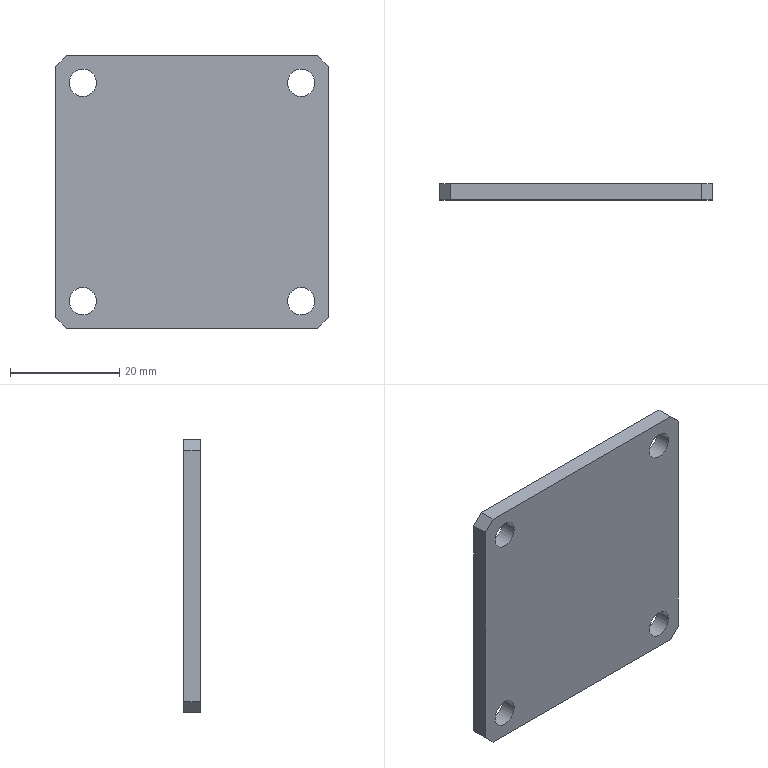Part | NX | 1 solid | 14 faces | box 50 x 3 x 50 mm | volume 7240 mm3 | plane 10 | cylinder 4 | commonest cylinder face diameters 5 x4
STEP:
#1=CARTESIAN_POINT('',(25.,3.,23.));
#2=VERTEX_POINT('',#1);
#3=CARTESIAN_POINT('',(25.,3.,-23.));
#4=VERTEX_POINT('',#3);
#5=CARTESIAN_POINT('',(25.,3.,25.));
#6=DIRECTION('',(0.,0.,-1.));
#7=VECTOR('',#6,1000.);
#8=LINE('',#5,#7);
#9=EDGE_CURVE('',#2,#4,#8,.T.);
#10=ORIENTED_EDGE('',*,*,#9,.F.);
#11=CARTESIAN_POINT('',(25.,0.,23.));
#12=VERTEX_POINT('',#11);
#13=CARTESIAN_POINT('',(25.,3.,23.));
#14=DIRECTION('',(0.,-1.,0.));
#15=VECTOR('',#14,1000.);
#16=LINE('',#13,#15);
#17=EDGE_CURVE('',#2,#12,#16,.T.);
#18=ORIENTED_EDGE('',*,*,#17,.T.);
#19=CARTESIAN_POINT('',(25.,0.,-23.));
#20=VERTEX_POINT('',#19);
#21=CARTESIAN_POINT('',(25.,0.,25.));
#22=DIRECTION('',(0.,0.,-1.));
#23=VECTOR('',#22,1000.);
#24=LINE('',#21,#23);
#25=EDGE_CURVE('',#12,#20,#24,.T.);
#26=ORIENTED_EDGE('',*,*,#25,.T.);
#27=CARTESIAN_POINT('',(25.,3.,-23.));
#28=DIRECTION('',(0.,1.,0.));
#29=VECTOR('',#28,1000.);
#30=LINE('',#27,#29);
#31=EDGE_CURVE('',#20,#4,#30,.T.);
#32=ORIENTED_EDGE('',*,*,#31,.T.);
#33=EDGE_LOOP('',(#10,#18,#26,#32));
#34=FACE_BOUND('',#33,.T.);
#35=CARTESIAN_POINT('',(25.,3.,25.));
#36=DIRECTION('',(-1.,0.,0.));
#37=DIRECTION('',(0.,0.,1.));
#38=AXIS2_PLACEMENT_3D('',#35,#36,#37);
#39=PLANE('',#38);
#40=ADVANCED_FACE('',(#34),#39,.F.);
#41=CARTESIAN_POINT('',(23.,3.,-25.));
#42=VERTEX_POINT('',#41);
#43=CARTESIAN_POINT('',(-23.,3.,-25.));
#44=VERTEX_POINT('',#43);
#45=CARTESIAN_POINT('',(-25.,3.,-25.));
#46=DIRECTION('',(-1.,0.,0.));
#47=VECTOR('',#46,1000.);
#48=LINE('',#45,#47);
#49=EDGE_CURVE('',#42,#44,#48,.T.);
#50=ORIENTED_EDGE('',*,*,#49,.F.);
#51=CARTESIAN_POINT('',(23.,0.,-25.));
#52=VERTEX_POINT('',#51);
#53=CARTESIAN_POINT('',(23.,3.,-25.));
#54=DIRECTION('',(0.,-1.,0.));
#55=VECTOR('',#54,1000.);
#56=LINE('',#53,#55);
#57=EDGE_CURVE('',#42,#52,#56,.T.);
#58=ORIENTED_EDGE('',*,*,#57,.T.);
#59=CARTESIAN_POINT('',(-23.,0.,-25.));
#60=VERTEX_POINT('',#59);
#61=CARTESIAN_POINT('',(-25.,0.,-25.));
#62=DIRECTION('',(-1.,0.,0.));
#63=VECTOR('',#62,1000.);
#64=LINE('',#61,#63);
#65=EDGE_CURVE('',#52,#60,#64,.T.);
#66=ORIENTED_EDGE('',*,*,#65,.T.);
#67=CARTESIAN_POINT('',(-23.,3.,-25.));
#68=DIRECTION('',(0.,1.,0.));
#69=VECTOR('',#68,1000.);
#70=LINE('',#67,#69);
#71=EDGE_CURVE('',#60,#44,#70,.T.);
#72=ORIENTED_EDGE('',*,*,#71,.T.);
#73=EDGE_LOOP('',(#50,#58,#66,#72));
#74=FACE_BOUND('',#73,.T.);
#75=CARTESIAN_POINT('',(-25.,3.,-25.));
#76=DIRECTION('',(0.,0.,1.));
#77=DIRECTION('',(1.,0.,0.));
#78=AXIS2_PLACEMENT_3D('',#75,#76,#77);
#79=PLANE('',#78);
#80=ADVANCED_FACE('',(#74),#79,.F.);
#81=CARTESIAN_POINT('',(-25.,0.,-23.));
#82=VERTEX_POINT('',#81);
#83=CARTESIAN_POINT('',(-25.,0.,23.));
#84=VERTEX_POINT('',#83);
#85=CARTESIAN_POINT('',(-25.,0.,25.));
#86=DIRECTION('',(0.,0.,1.));
#87=VECTOR('',#86,1000.);
#88=LINE('',#85,#87);
#89=EDGE_CURVE('',#82,#84,#88,.T.);
#90=ORIENTED_EDGE('',*,*,#89,.T.);
#91=CARTESIAN_POINT('',(-25.,3.,23.));
#92=VERTEX_POINT('',#91);
#93=CARTESIAN_POINT('',(-25.,3.,23.));
#94=DIRECTION('',(0.,1.,0.));
#95=VECTOR('',#94,1000.);
#96=LINE('',#93,#95);
#97=EDGE_CURVE('',#84,#92,#96,.T.);
#98=ORIENTED_EDGE('',*,*,#97,.T.);
#99=CARTESIAN_POINT('',(-25.,3.,-23.));
#100=VERTEX_POINT('',#99);
#101=CARTESIAN_POINT('',(-25.,3.,25.));
#102=DIRECTION('',(0.,0.,1.));
#103=VECTOR('',#102,1000.);
#104=LINE('',#101,#103);
#105=EDGE_CURVE('',#100,#92,#104,.T.);
#106=ORIENTED_EDGE('',*,*,#105,.F.);
#107=CARTESIAN_POINT('',(-25.,3.,-23.));
#108=DIRECTION('',(0.,-1.,0.));
#109=VECTOR('',#108,1000.);
#110=LINE('',#107,#109);
#111=EDGE_CURVE('',#100,#82,#110,.T.);
#112=ORIENTED_EDGE('',*,*,#111,.T.);
#113=EDGE_LOOP('',(#90,#98,#106,#112));
#114=FACE_BOUND('',#113,.T.);
#115=CARTESIAN_POINT('',(-25.,3.,25.));
#116=DIRECTION('',(1.,0.,0.));
#117=DIRECTION('',(0.,0.,-1.));
#118=AXIS2_PLACEMENT_3D('',#115,#116,#117);
#119=PLANE('',#118);
#120=ADVANCED_FACE('',(#114),#119,.F.);
#121=CARTESIAN_POINT('',(-23.,3.,25.));
#122=VERTEX_POINT('',#121);
#123=CARTESIAN_POINT('',(23.,3.,25.));
#124=VERTEX_POINT('',#123);
#125=CARTESIAN_POINT('',(-25.,3.,25.));
#126=DIRECTION('',(1.,0.,0.));
#127=VECTOR('',#126,1000.);
#128=LINE('',#125,#127);
#129=EDGE_CURVE('',#122,#124,#128,.T.);
#130=ORIENTED_EDGE('',*,*,#129,.F.);
#131=CARTESIAN_POINT('',(-23.,0.,25.));
#132=VERTEX_POINT('',#131);
#133=CARTESIAN_POINT('',(-23.,3.,25.));
#134=DIRECTION('',(0.,-1.,0.));
#135=VECTOR('',#134,1000.);
#136=LINE('',#133,#135);
#137=EDGE_CURVE('',#122,#132,#136,.T.);
#138=ORIENTED_EDGE('',*,*,#137,.T.);
#139=CARTESIAN_POINT('',(23.,0.,25.));
#140=VERTEX_POINT('',#139);
#141=CARTESIAN_POINT('',(-25.,0.,25.));
#142=DIRECTION('',(1.,0.,0.));
#143=VECTOR('',#142,1000.);
#144=LINE('',#141,#143);
#145=EDGE_CURVE('',#132,#140,#144,.T.);
#146=ORIENTED_EDGE('',*,*,#145,.T.);
#147=CARTESIAN_POINT('',(23.,3.,25.));
#148=DIRECTION('',(0.,1.,0.));
#149=VECTOR('',#148,1000.);
#150=LINE('',#147,#149);
#151=EDGE_CURVE('',#140,#124,#150,.T.);
#152=ORIENTED_EDGE('',*,*,#151,.T.);
#153=EDGE_LOOP('',(#130,#138,#146,#152));
#154=FACE_BOUND('',#153,.T.);
#155=CARTESIAN_POINT('',(-25.,3.,25.));
#156=DIRECTION('',(0.,0.,-1.));
#157=DIRECTION('',(-1.,0.,0.));
#158=AXIS2_PLACEMENT_3D('',#155,#156,#157);
#159=PLANE('',#158);
#160=ADVANCED_FACE('',(#154),#159,.F.);
#161=CARTESIAN_POINT('',(-20.,3.,-17.5));
#162=VERTEX_POINT('',#161);
#163=CARTESIAN_POINT('',(-20.,3.,-20.));
#164=DIRECTION('',(0.,1.,0.));
#165=DIRECTION('',(0.,0.,1.));
#166=AXIS2_PLACEMENT_3D('',#163,#164,#165);
#167=CIRCLE('',#166,2.5);
#168=EDGE_CURVE('',#162,#162,#167,.T.);
#169=ORIENTED_EDGE('',*,*,#168,.F.);
#170=EDGE_LOOP('',(#169));
#171=FACE_BOUND('',#170,.T.);
#172=CARTESIAN_POINT('',(20.,3.,-17.5));
#173=VERTEX_POINT('',#172);
#174=CARTESIAN_POINT('',(20.,3.,-20.));
#175=DIRECTION('',(0.,1.,0.));
#176=DIRECTION('',(0.,0.,1.));
#177=AXIS2_PLACEMENT_3D('',#174,#175,#176);
#178=CIRCLE('',#177,2.5);
#179=EDGE_CURVE('',#173,#173,#178,.T.);
#180=ORIENTED_EDGE('',*,*,#179,.F.);
#181=EDGE_LOOP('',(#180));
#182=FACE_BOUND('',#181,.T.);
#183=CARTESIAN_POINT('',(20.,3.,22.5));
#184=VERTEX_POINT('',#183);
#185=CARTESIAN_POINT('',(20.,3.,20.));
#186=DIRECTION('',(0.,1.,0.));
#187=DIRECTION('',(0.,0.,1.));
#188=AXIS2_PLACEMENT_3D('',#185,#186,#187);
#189=CIRCLE('',#188,2.5);
#190=EDGE_CURVE('',#184,#184,#189,.T.);
#191=ORIENTED_EDGE('',*,*,#190,.F.);
#192=EDGE_LOOP('',(#191));
#193=FACE_BOUND('',#192,.T.);
#194=CARTESIAN_POINT('',(-20.,3.,22.5));
#195=VERTEX_POINT('',#194);
#196=CARTESIAN_POINT('',(-20.,3.,20.));
#197=DIRECTION('',(0.,1.,0.));
#198=DIRECTION('',(0.,0.,1.));
#199=AXIS2_PLACEMENT_3D('',#196,#197,#198);
#200=CIRCLE('',#199,2.5);
#201=EDGE_CURVE('',#195,#195,#200,.T.);
#202=ORIENTED_EDGE('',*,*,#201,.F.);
#203=EDGE_LOOP('',(#202));
#204=FACE_BOUND('',#203,.T.);
#205=ORIENTED_EDGE('',*,*,#105,.T.);
#206=CARTESIAN_POINT('',(-23.,3.,25.));
#207=DIRECTION('',(-0.7071,0.,-0.7071));
#208=VECTOR('',#207,1000.);
#209=LINE('',#206,#208);
#210=EDGE_CURVE('',#92,#122,#209,.F.);
#211=ORIENTED_EDGE('',*,*,#210,.T.);
#212=ORIENTED_EDGE('',*,*,#129,.T.);
#213=CARTESIAN_POINT('',(25.,3.,23.));
#214=DIRECTION('',(-0.7071,0.,0.7071));
#215=VECTOR('',#214,1000.);
#216=LINE('',#213,#215);
#217=EDGE_CURVE('',#124,#2,#216,.F.);
#218=ORIENTED_EDGE('',*,*,#217,.T.);
#219=ORIENTED_EDGE('',*,*,#9,.T.);
#220=CARTESIAN_POINT('',(23.,3.,-25.));
#221=DIRECTION('',(0.7071,0.,0.7071));
#222=VECTOR('',#221,1000.);
#223=LINE('',#220,#222);
#224=EDGE_CURVE('',#4,#42,#223,.F.);
#225=ORIENTED_EDGE('',*,*,#224,.T.);
#226=ORIENTED_EDGE('',*,*,#49,.T.);
#227=CARTESIAN_POINT('',(-25.,3.,-23.));
#228=DIRECTION('',(0.7071,0.,-0.7071));
#229=VECTOR('',#228,1000.);
#230=LINE('',#227,#229);
#231=EDGE_CURVE('',#44,#100,#230,.F.);
#232=ORIENTED_EDGE('',*,*,#231,.T.);
#233=EDGE_LOOP('',(#205,#211,#212,#218,#219,#225,#226,#232));
#234=FACE_BOUND('',#233,.T.);
#235=CARTESIAN_POINT('',(0.,3.,0.));
#236=DIRECTION('',(0.,-1.,0.));
#237=DIRECTION('',(0.,0.,-1.));
#238=AXIS2_PLACEMENT_3D('',#235,#236,#237);
#239=PLANE('',#238);
#240=ADVANCED_FACE('',(#171,#182,#193,#204,#234),#239,.F.);
#241=CARTESIAN_POINT('',(-20.,0.,-17.5));
#242=VERTEX_POINT('',#241);
#243=CARTESIAN_POINT('',(-20.,0.,-20.));
#244=DIRECTION('',(0.,1.,0.));
#245=DIRECTION('',(0.,0.,1.));
#246=AXIS2_PLACEMENT_3D('',#243,#244,#245);
#247=CIRCLE('',#246,2.5);
#248=EDGE_CURVE('',#242,#242,#247,.T.);
#249=ORIENTED_EDGE('',*,*,#248,.T.);
#250=EDGE_LOOP('',(#249));
#251=FACE_BOUND('',#250,.T.);
#252=CARTESIAN_POINT('',(20.,0.,-17.5));
#253=VERTEX_POINT('',#252);
#254=CARTESIAN_POINT('',(20.,0.,-20.));
#255=DIRECTION('',(0.,1.,0.));
#256=DIRECTION('',(0.,0.,1.));
#257=AXIS2_PLACEMENT_3D('',#254,#255,#256);
#258=CIRCLE('',#257,2.5);
#259=EDGE_CURVE('',#253,#253,#258,.T.);
#260=ORIENTED_EDGE('',*,*,#259,.T.);
#261=EDGE_LOOP('',(#260));
#262=FACE_BOUND('',#261,.T.);
#263=CARTESIAN_POINT('',(20.,0.,22.5));
#264=VERTEX_POINT('',#263);
#265=CARTESIAN_POINT('',(20.,0.,20.));
#266=DIRECTION('',(0.,1.,0.));
#267=DIRECTION('',(0.,0.,1.));
#268=AXIS2_PLACEMENT_3D('',#265,#266,#267);
#269=CIRCLE('',#268,2.5);
#270=EDGE_CURVE('',#264,#264,#269,.T.);
#271=ORIENTED_EDGE('',*,*,#270,.T.);
#272=EDGE_LOOP('',(#271));
#273=FACE_BOUND('',#272,.T.);
#274=CARTESIAN_POINT('',(-20.,0.,22.5));
#275=VERTEX_POINT('',#274);
#276=CARTESIAN_POINT('',(-20.,0.,20.));
#277=DIRECTION('',(0.,1.,0.));
#278=DIRECTION('',(0.,0.,1.));
#279=AXIS2_PLACEMENT_3D('',#276,#277,#278);
#280=CIRCLE('',#279,2.5);
#281=EDGE_CURVE('',#275,#275,#280,.T.);
#282=ORIENTED_EDGE('',*,*,#281,.T.);
#283=EDGE_LOOP('',(#282));
#284=FACE_BOUND('',#283,.T.);
#285=ORIENTED_EDGE('',*,*,#145,.F.);
#286=CARTESIAN_POINT('',(-24.,0.,24.));
#287=DIRECTION('',(0.7071,0.,0.7071));
#288=VECTOR('',#287,1000.);
#289=LINE('',#286,#288);
#290=EDGE_CURVE('',#132,#84,#289,.F.);
#291=ORIENTED_EDGE('',*,*,#290,.T.);
#292=ORIENTED_EDGE('',*,*,#89,.F.);
#293=CARTESIAN_POINT('',(-24.,0.,-24.));
#294=DIRECTION('',(-0.7071,0.,0.7071));
#295=VECTOR('',#294,1000.);
#296=LINE('',#293,#295);
#297=EDGE_CURVE('',#82,#60,#296,.F.);
#298=ORIENTED_EDGE('',*,*,#297,.T.);
#299=ORIENTED_EDGE('',*,*,#65,.F.);
#300=CARTESIAN_POINT('',(24.,0.,-24.));
#301=DIRECTION('',(-0.7071,0.,-0.7071));
#302=VECTOR('',#301,1000.);
#303=LINE('',#300,#302);
#304=EDGE_CURVE('',#52,#20,#303,.F.);
#305=ORIENTED_EDGE('',*,*,#304,.T.);
#306=ORIENTED_EDGE('',*,*,#25,.F.);
#307=CARTESIAN_POINT('',(24.,0.,24.));
#308=DIRECTION('',(0.7071,0.,-0.7071));
#309=VECTOR('',#308,1000.);
#310=LINE('',#307,#309);
#311=EDGE_CURVE('',#12,#140,#310,.F.);
#312=ORIENTED_EDGE('',*,*,#311,.T.);
#313=EDGE_LOOP('',(#285,#291,#292,#298,#299,#305,#306,#312));
#314=FACE_BOUND('',#313,.T.);
#315=CARTESIAN_POINT('',(0.,0.,0.));
#316=DIRECTION('',(0.,-1.,0.));
#317=DIRECTION('',(0.,0.,-1.));
#318=AXIS2_PLACEMENT_3D('',#315,#316,#317);
#319=PLANE('',#318);
#320=ADVANCED_FACE('',(#251,#262,#273,#284,#314),#319,.T.);
#321=ORIENTED_EDGE('',*,*,#210,.F.);
#322=ORIENTED_EDGE('',*,*,#97,.F.);
#323=ORIENTED_EDGE('',*,*,#290,.F.);
#324=ORIENTED_EDGE('',*,*,#137,.F.);
#325=EDGE_LOOP('',(#321,#322,#323,#324));
#326=FACE_BOUND('',#325,.T.);
#327=CARTESIAN_POINT('',(-23.,3.,25.));
#328=DIRECTION('',(0.7071,0.,-0.7071));
#329=DIRECTION('',(0.,-1.,0.));
#330=AXIS2_PLACEMENT_3D('',#327,#328,#329);
#331=PLANE('',#330);
#332=ADVANCED_FACE('',(#326),#331,.F.);
#333=ORIENTED_EDGE('',*,*,#217,.F.);
#334=ORIENTED_EDGE('',*,*,#151,.F.);
#335=ORIENTED_EDGE('',*,*,#311,.F.);
#336=ORIENTED_EDGE('',*,*,#17,.F.);
#337=EDGE_LOOP('',(#333,#334,#335,#336));
#338=FACE_BOUND('',#337,.T.);
#339=CARTESIAN_POINT('',(25.,3.,23.));
#340=DIRECTION('',(-0.7071,0.,-0.7071));
#341=DIRECTION('',(0.,-1.,0.));
#342=AXIS2_PLACEMENT_3D('',#339,#340,#341);
#343=PLANE('',#342);
#344=ADVANCED_FACE('',(#338),#343,.F.);
#345=ORIENTED_EDGE('',*,*,#224,.F.);
#346=ORIENTED_EDGE('',*,*,#31,.F.);
#347=ORIENTED_EDGE('',*,*,#304,.F.);
#348=ORIENTED_EDGE('',*,*,#57,.F.);
#349=EDGE_LOOP('',(#345,#346,#347,#348));
#350=FACE_BOUND('',#349,.T.);
#351=CARTESIAN_POINT('',(23.,3.,-25.));
#352=DIRECTION('',(-0.7071,0.,0.7071));
#353=DIRECTION('',(0.,-1.,0.));
#354=AXIS2_PLACEMENT_3D('',#351,#352,#353);
#355=PLANE('',#354);
#356=ADVANCED_FACE('',(#350),#355,.F.);
#357=ORIENTED_EDGE('',*,*,#231,.F.);
#358=ORIENTED_EDGE('',*,*,#71,.F.);
#359=ORIENTED_EDGE('',*,*,#297,.F.);
#360=ORIENTED_EDGE('',*,*,#111,.F.);
#361=EDGE_LOOP('',(#357,#358,#359,#360));
#362=FACE_BOUND('',#361,.T.);
#363=CARTESIAN_POINT('',(-25.,3.,-23.));
#364=DIRECTION('',(0.7071,0.,0.7071));
#365=DIRECTION('',(0.,-1.,0.));
#366=AXIS2_PLACEMENT_3D('',#363,#364,#365);
#367=PLANE('',#366);
#368=ADVANCED_FACE('',(#362),#367,.F.);
#369=ORIENTED_EDGE('',*,*,#281,.F.);
#370=EDGE_LOOP('',(#369));
#371=FACE_BOUND('',#370,.T.);
#372=ORIENTED_EDGE('',*,*,#201,.T.);
#373=EDGE_LOOP('',(#372));
#374=FACE_BOUND('',#373,.T.);
#375=CARTESIAN_POINT('',(-20.,3.,20.));
#376=DIRECTION('',(0.,1.,0.));
#377=DIRECTION('',(0.,0.,1.));
#378=AXIS2_PLACEMENT_3D('',#375,#376,#377);
#379=CYLINDRICAL_SURFACE('',#378,2.5);
#380=ADVANCED_FACE('',(#371,#374),#379,.F.);
#381=ORIENTED_EDGE('',*,*,#270,.F.);
#382=EDGE_LOOP('',(#381));
#383=FACE_BOUND('',#382,.T.);
#384=ORIENTED_EDGE('',*,*,#190,.T.);
#385=EDGE_LOOP('',(#384));
#386=FACE_BOUND('',#385,.T.);
#387=CARTESIAN_POINT('',(20.,3.,20.));
#388=DIRECTION('',(0.,1.,0.));
#389=DIRECTION('',(0.,0.,1.));
#390=AXIS2_PLACEMENT_3D('',#387,#388,#389);
#391=CYLINDRICAL_SURFACE('',#390,2.5);
#392=ADVANCED_FACE('',(#383,#386),#391,.F.);
#393=ORIENTED_EDGE('',*,*,#259,.F.);
#394=EDGE_LOOP('',(#393));
#395=FACE_BOUND('',#394,.T.);
#396=ORIENTED_EDGE('',*,*,#179,.T.);
#397=EDGE_LOOP('',(#396));
#398=FACE_BOUND('',#397,.T.);
#399=CARTESIAN_POINT('',(20.,3.,-20.));
#400=DIRECTION('',(0.,1.,0.));
#401=DIRECTION('',(0.,0.,1.));
#402=AXIS2_PLACEMENT_3D('',#399,#400,#401);
#403=CYLINDRICAL_SURFACE('',#402,2.5);
#404=ADVANCED_FACE('',(#395,#398),#403,.F.);
#405=ORIENTED_EDGE('',*,*,#248,.F.);
#406=EDGE_LOOP('',(#405));
#407=FACE_BOUND('',#406,.T.);
#408=ORIENTED_EDGE('',*,*,#168,.T.);
#409=EDGE_LOOP('',(#408));
#410=FACE_BOUND('',#409,.T.);
#411=CARTESIAN_POINT('',(-20.,3.,-20.));
#412=DIRECTION('',(0.,1.,0.));
#413=DIRECTION('',(0.,0.,1.));
#414=AXIS2_PLACEMENT_3D('',#411,#412,#413);
#415=CYLINDRICAL_SURFACE('',#414,2.5);
#416=ADVANCED_FACE('',(#407,#410),#415,.F.);
#417=CLOSED_SHELL('',(#40,#80,#120,#160,#240,#320,#332,#344,#356,#368,#380,#392,#404,#416));
#418=MANIFOLD_SOLID_BREP('',#417);
#419=(LENGTH_UNIT()NAMED_UNIT(*)SI_UNIT(.MILLI.,.METRE.));
#420=UNCERTAINTY_MEASURE_WITH_UNIT(LENGTH_MEASURE(0.00001),#419,'','');
#421=(NAMED_UNIT(*)PLANE_ANGLE_UNIT()SI_UNIT($,.RADIAN.));
#422=(NAMED_UNIT(*)SI_UNIT($,.STERADIAN.)SOLID_ANGLE_UNIT());
#423=(GEOMETRIC_REPRESENTATION_CONTEXT(3)GLOBAL_UNCERTAINTY_ASSIGNED_CONTEXT((#420))GLOBAL_UNIT_ASSIGNED_CONTEXT((#419,#421,#422))REPRESENTATION_CONTEXT('',''));
#424=ADVANCED_BREP_SHAPE_REPRESENTATION('',(#418),#423);